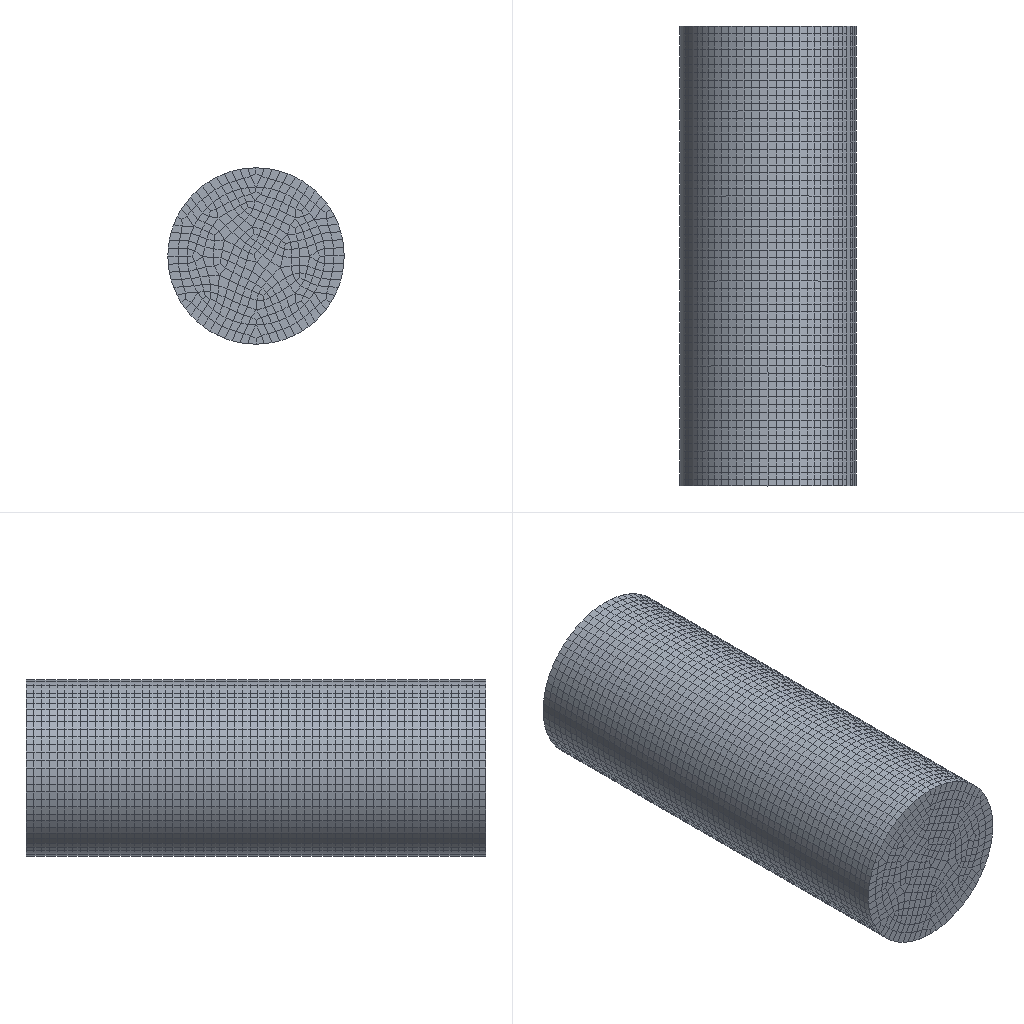Simulation study | ansys workbench
Ansys APDL input file, long lists of numbers shortened:
/batch
/config,noeldb,1     ! force off writing results to database
*get,_wallstrt,active,,time,wall
! ANSYS input file written by Workbench version 2020 R2
! File used for geometry attach:
/title,unsaved_project--___ 2 (C5)
*DIM,_wb_ProjectScratch_dir,string,248
_wb_ProjectScratch_dir(1) = ''
*DIM,_wb_SolverFiles_dir,string,248
_wb_SolverFiles_dir(1) = ''
*DIM,_wb_userfiles_dir,string,248
_wb_userfiles_dir(1) = ''
/com,--- Data in consistent MKS units. See Solving Units in the help system for more information.
/units,MKS
/nopr
/wb,file,start              !  signify a WB generated input file
/prep7
! Turn off shape checking because checks already performed inside WB mesher.
! See help system for more information.
SHPP,OFF,,NOWARN
/nolist
etcon,set             ! allow ANSYS to choose best KEYOP's for 180x elements
/com,*********** Nodes for the whole assembly ***********
nblock,3,,50740
(1i9,3e20.9e3)
        1    -1.192148224E-02     0.000000000E+00    -1.104059469E-02
! (46127 more lines like these left out)
-1
/wb,elem,start            !  set before creation of elements
/com,*********** Elements for Body 1 "SYS\__" ***********
et,1,90
eblock,19,solid,,8511
(19i9)
        1        1        1        1        0        0        0        0       20        0        1      424      532    12288    12285      422      531    12424    12421
! (17021 more lines like these left out)
-1
/wb,elem,end               !  done creating elements
/com,*********** Send User Defined Coordinate System(s) ***********
csys,0
toffst,273.15,  ! Temperature offset from absolute zero
/wb,mat,start              !  starting to send materials
/com,*********** Send Materials ***********
Temperature = 'TEMP' ! Temperature
MP,DENS,1,7850,	! kg m^-3
MP,ALPX,1,1.2e-05,	! C^-1
MP,C,1,434,	! J kg^-1 C^-1
MP,KXX,1,60.5,	! W m^-1 C^-1
MP,RSVX,1,1.7e-07,	! kg m^3 A^-2 s^-3
MP,EX,1,200000000000,	! Pa
MP,NUXY,1,0.3,
MP,MURX,1,10000,
/wb,mat,end                !  done sending materials
!************************* Model Summary ********************
!SYS\__,	Structural Steel,	matid,	1
!************************* End Model Summary ********************
! get the diagonal of the bounding box. Needed later for other things
*get,_xmin,node,,mnloc,x
*get,_ymin,node,,mnloc,y
*get,_zmin,node,,mnloc,z
*get,_xmax,node,,mxloc,x
*get,_ymax,node,,mxloc,y
*get,_zmax,node,,mxloc,z
_ASMDIAG=(_xmax-_xmin)*(_xmax-_xmin)+(_ymax-_ymin)*(_ymax-_ymin)+(_zmax-_zmin)*(_zmax-_zmin)
_ASMDIAG=SQRT(_ASMDIAG)
/wb,contact,start          !  starting to send contact
/wb,contact,end            !  done creating contacts
/golist
/wb,load,start             !  starting to send loads
fcum,add                   ! add nodal forces up (needed in case have loads on the same edge,vertex)
fcum                       ! reset default on fcum command since done sending WB F loads
/com,*********** Create "______" ***********
et,2,152
eblock,10,,,4080
(15i9)
    16518        2        2        2        0    12215    12217    12081    12079    45179    45178    44727    45173
! (4079 more lines like these left out)
-1
esel,s,type,,2
keyop,2,8,2.
keyop,2,13,0
esel,all
/com,*********** Send Solved Initial Temperatures ***********
/nopr
ic,1,temp,99.381
ic,2,temp,99.286
ic,3,temp,99.555
ic,4,temp,99.382
! (46124 more lines like these left out)
/gopr
/gst,on,on
fini
*get,_numnode,node,0,count
*get,_numelem,elem,0,count
*get, _MAXELEMNUM, elem, 0, NUM, MAX
*get, _MAXNODENUM, node, 0, NUM, MAX
*get, _MAXELEMTYPE, etyp, 0, NUM, MAX
*get, _MAXREALCONST, real, 0, NUM, MAX
/go
/wb,load,end               !  done creating loads
/com,--- Number of total nodes = %_numnode%
/com,--- Number of contact elements = 4080
/com,--- Number of spring elements = 0
/com,--- Number of bearing elements = 0
/com,--- Number of solid elements = 8511
/com,--- Number of condensed parts = 0
/com,--- Number of total elements = %_numelem%
*get,_wallbsol,active,,time,wall
/com,****************************************************************************
/com,*************************    SOLUTION       ********************************
/com,****************************************************************************
/solu
antype,4                   ! transient analysis
kbc,1                      ! stepped BC's
!eqsl,sparse               ! using sparse solver which is default so no eqsl command needed
cntr,print,1               ! print out contact info and also make no initial contact an error
rescontrol,,none                 ! Do not keep any restart files
thopt,quasi,5.e-002
nlhist,nsol,MAX_TEMP,temp,max
nlhist,nsol,MIN_TEMP,temp,min
/com,********* Initial Time Increment Check And Fourier Modulus *********
/com, Specified Initial Time Increment: 1
/com, Estimated Increment Needed, le*le/alpha, Body 1: 0.2533
/com,****************************************************
/com,******************* SOLVE FOR LS 1 OF 1 ****************
esel,s,type,,2
nsle
sf,all,conv,250.,22.
nsel,all
esel,all
autots,on
nsub,100,1000,10
time,100.
timint,on                  ! Turn on time integration effects
outres,erase
outres,all,none
outres,nsol,all
outres,rsol,all
outres,eangl,all
outres,veng,all
outres,fflux,all
outres,cont,all
/nopr
esel,s,type,,2
cm,_elmisc,elem
esel,all
/gopr
outres,misc,all,_elmisc
cnvtol,heat,,.001,,1.e-006    ! Program Controlled. Set MINREF equivalent of 1e-6 Watts
! *********** WB SOLVE COMMAND ***********
! check interactive state
*get,ANSINTER_,active,,int
*if,ANSINTER_,ne,0,then
/eof
*endif
solve
/com *************** Write FE CONNECTORS *********
CEWRITE,file,ce,,INTE
/com,****************************************************
/com,*************** FINISHED SOLVE FOR LS 1 *************
*get,_wallasol,active,,time,wall
/post1
xmlo,ENCODING,ISO-8859-1
xmlo,parm
/xml,parm,xml
fini
/gopr
*get,_walldone,active,,time,wall
_preptime=(_wallbsol-_wallstrt)*3600
_solvtime=(_wallasol-_wallbsol)*3600
_posttime=(_walldone-_wallasol)*3600
_totaltim=(_walldone-_wallstrt)*3600
*get,_dlbratio,active,0,solu,dlbr
*get,_combtime,active,0,solu,comb
/com,--- Total number of nodes = %_numnode%
/com,--- Total number of elements = %_numelem%
/com,--- Element load balance ratio = %_dlbratio%
/com,--- Time to combine distributed files = %_combtime%
/wb,file,end               ! done with WB generated input